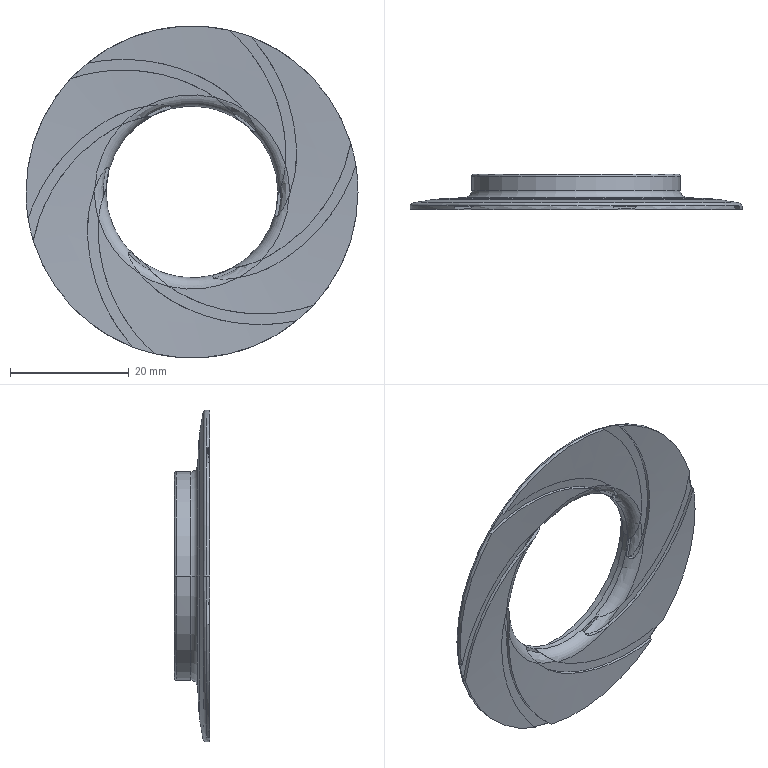Part | STEP file | DW-T1-02-0032_2_1_1 | 1 solid | 101 faces | box 56 x 5.906 x 56 mm | volume 3121 mm3 | cylinder 50 | cone 18 | torus 17 | plane 10 | other 6 | commonest cylinder face diameters 34.8 x12 21.61 x6 38.382 x6 38.4 x6 56.8 x6 60.4 x6